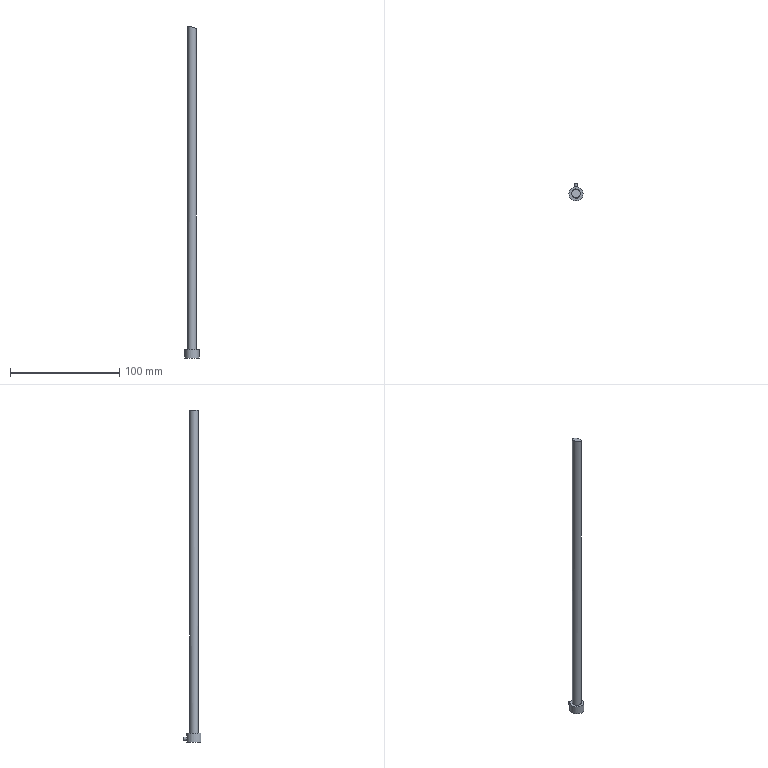Part | STEP file | E108-07-310 | 1 solid | 8 faces | box 13 x 16.5 x 303.697 mm | volume 15889 mm3 | cylinder 3 | plane 3 | spline 1 | cone 1 | commonest cylinder face diameters 3 x1 8 x1 13 x1
STEP:
#1=CARTESIAN_POINT('',(0.,0.,0.));
#2=DIRECTION('',(0.,0.,1.));
#3=DIRECTION('',(1.,0.,0.));
#4=AXIS2_PLACEMENT_3D('',#1,#2,#3);
#5=CARTESIAN_POINT('',(3.981,0.3919,301.273));
#6=VERTEX_POINT('',#5);
#7=CARTESIAN_POINT('',(3.981,0.3919,301.273));
#8=CARTESIAN_POINT('',(3.938,0.8228,301.273));
#9=CARTESIAN_POINT('',(3.823,1.252,301.297));
#10=CARTESIAN_POINT('',(3.646,1.645,301.341));
#11=CARTESIAN_POINT('',(3.469,2.037,301.385));
#12=CARTESIAN_POINT('',(3.225,2.404,301.45));
#13=CARTESIAN_POINT('',(2.937,2.716,301.53));
#14=CARTESIAN_POINT('',(2.642,3.034,301.612));
#15=CARTESIAN_POINT('',(2.293,3.305,301.711));
#16=CARTESIAN_POINT('',(1.918,3.51,301.82));
#17=CARTESIAN_POINT('',(1.526,3.724,301.934));
#18=CARTESIAN_POINT('',(1.096,3.872,302.061));
#19=CARTESIAN_POINT('',(0.6599,3.945,302.191));
#20=CARTESIAN_POINT('',(0.2071,4.021,302.327));
#21=CARTESIAN_POINT('',(-0.2637,4.018,302.469));
#22=CARTESIAN_POINT('',(-0.7148,3.936,302.606));
#23=CARTESIAN_POINT('',(-1.175,3.852,302.747));
#24=CARTESIAN_POINT('',(-1.627,3.685,302.886));
#25=CARTESIAN_POINT('',(-2.032,3.445,303.013));
#26=CARTESIAN_POINT('',(-2.434,3.208,303.139));
#27=CARTESIAN_POINT('',(-2.802,2.893,303.257));
#28=CARTESIAN_POINT('',(-3.101,2.526,303.355));
#29=CARTESIAN_POINT('',(-3.39,2.171,303.45));
#30=CARTESIAN_POINT('',(-3.623,1.757,303.531));
#31=CARTESIAN_POINT('',(-3.776,1.319,303.588));
#32=CARTESIAN_POINT('',(-3.923,0.8987,303.643));
#33=CARTESIAN_POINT('',(-4.,0.4448,303.678));
#34=CARTESIAN_POINT('',(-4.,-0.003275,303.691));
#35=CARTESIAN_POINT('',(-4.,-0.4371,303.703));
#36=CARTESIAN_POINT('',(-3.927,-0.8775,303.695));
#37=CARTESIAN_POINT('',(-3.787,-1.287,303.666));
#38=CARTESIAN_POINT('',(-3.649,-1.694,303.637));
#39=CARTESIAN_POINT('',(-3.442,-2.081,303.588));
#40=CARTESIAN_POINT('',(-3.185,-2.42,303.522));
#41=CARTESIAN_POINT('',(-2.924,-2.764,303.455));
#42=CARTESIAN_POINT('',(-2.604,-3.066,303.369));
#43=CARTESIAN_POINT('',(-2.251,-3.306,303.272));
#44=CARTESIAN_POINT('',(-1.886,-3.555,303.171));
#45=CARTESIAN_POINT('',(-1.478,-3.743,303.055));
#46=CARTESIAN_POINT('',(-1.057,-3.858,302.932));
#47=CARTESIAN_POINT('',(-0.6196,-3.978,302.805));
#48=CARTESIAN_POINT('',(-0.1578,-4.022,302.667));
#49=CARTESIAN_POINT('',(0.2919,-3.989,302.53));
#50=CARTESIAN_POINT('',(0.7551,-3.955,302.389));
#51=CARTESIAN_POINT('',(1.218,-3.838,302.245));
#52=CARTESIAN_POINT('',(1.643,-3.647,302.109));
#53=CARTESIAN_POINT('',(2.07,-3.454,301.973));
#54=CARTESIAN_POINT('',(2.471,-3.181,301.842));
#55=CARTESIAN_POINT('',(2.809,-2.848,301.729));
#56=CARTESIAN_POINT('',(3.138,-2.523,301.618));
#57=CARTESIAN_POINT('',(3.417,-2.131,301.52));
#58=CARTESIAN_POINT('',(3.618,-1.706,301.445));
#59=CARTESIAN_POINT('',(3.81,-1.3,301.374));
#60=CARTESIAN_POINT('',(3.935,-0.8505,301.322));
#61=CARTESIAN_POINT('',(3.98,-0.3986,301.295));
#62=CARTESIAN_POINT('',(4.006,-0.1368,301.28));
#63=CARTESIAN_POINT('',(4.007,0.1295,301.272));
#64=CARTESIAN_POINT('',(3.981,0.3919,301.273));
#65=B_SPLINE_CURVE_WITH_KNOTS('',3,(#7,#8,#9,#10,#11,#12,#13,#14,#15,#16,#17,#18,#19,#20,#21,#22,#23,#24,#25,#26,#27,#28,#29,#30,#31,#32,#33,#34,#35,#36,#37,#38,#39,#40,#41,#42,#43,#44,#45,#46,#47,#48,#49,#50,#51,#52,#53,#54,#55,#56,#57,#58,#59,#60,#61,#62,#63,#64),.UNSPECIFIED.,.T.,.F.,(1,3,3,3,3,3,3,3,3,3,3,3,3,3,3,3,3,3,3,3,3,1),(-0.03062,0.,0.05078,0.1015,0.1532,0.2072,0.2634,0.3207,0.3774,0.4324,0.485,0.5359,0.5863,0.6375,0.6906,0.7458,0.8028,0.8601,0.916,0.9694,1.,1.051),.UNSPECIFIED.);
#66=CARTESIAN_POINT('',(0.,0.,108.));
#67=DIRECTION('',(0.,0.,-1.));
#68=DIRECTION('',(-1.,0.,0.));
#69=AXIS2_PLACEMENT_3D('',#66,#67,#68);
#70=CYLINDRICAL_SURFACE('',#69,4.);
#71=CARTESIAN_POINT('',(9.327,-193.273));
#72=CARTESIAN_POINT('',(9.302,-193.273));
#73=CARTESIAN_POINT('',(9.254,-193.275));
#74=CARTESIAN_POINT('',(9.181,-193.286));
#75=CARTESIAN_POINT('',(9.108,-193.303));
#76=CARTESIAN_POINT('',(9.035,-193.327));
#77=CARTESIAN_POINT('',(8.962,-193.356));
#78=CARTESIAN_POINT('',(8.89,-193.392));
#79=CARTESIAN_POINT('',(8.817,-193.434));
#80=CARTESIAN_POINT('',(8.745,-193.481));
#81=CARTESIAN_POINT('',(8.674,-193.533));
#82=CARTESIAN_POINT('',(8.602,-193.589));
#83=CARTESIAN_POINT('',(8.53,-193.651));
#84=CARTESIAN_POINT('',(8.459,-193.716));
#85=CARTESIAN_POINT('',(8.388,-193.785));
#86=CARTESIAN_POINT('',(8.318,-193.857));
#87=CARTESIAN_POINT('',(8.247,-193.933));
#88=CARTESIAN_POINT('',(8.177,-194.011));
#89=CARTESIAN_POINT('',(8.106,-194.09));
#90=CARTESIAN_POINT('',(8.036,-194.172));
#91=CARTESIAN_POINT('',(7.966,-194.254));
#92=CARTESIAN_POINT('',(7.896,-194.338));
#93=CARTESIAN_POINT('',(7.826,-194.423));
#94=CARTESIAN_POINT('',(7.756,-194.507));
#95=CARTESIAN_POINT('',(7.687,-194.592));
#96=CARTESIAN_POINT('',(7.617,-194.675));
#97=CARTESIAN_POINT('',(7.547,-194.758));
#98=CARTESIAN_POINT('',(7.477,-194.839));
#99=CARTESIAN_POINT('',(7.406,-194.919));
#100=CARTESIAN_POINT('',(7.336,-194.997));
#101=CARTESIAN_POINT('',(7.266,-195.072));
#102=CARTESIAN_POINT('',(7.195,-195.145));
#103=CARTESIAN_POINT('',(7.124,-195.215));
#104=CARTESIAN_POINT('',(7.053,-195.281));
#105=CARTESIAN_POINT('',(6.982,-195.343));
#106=CARTESIAN_POINT('',(6.911,-195.401));
#107=CARTESIAN_POINT('',(6.839,-195.455));
#108=CARTESIAN_POINT('',(6.767,-195.504));
#109=CARTESIAN_POINT('',(6.695,-195.548));
#110=CARTESIAN_POINT('',(6.623,-195.587));
#111=CARTESIAN_POINT('',(6.55,-195.62));
#112=CARTESIAN_POINT('',(6.478,-195.648));
#113=CARTESIAN_POINT('',(6.405,-195.669));
#114=CARTESIAN_POINT('',(6.332,-195.685));
#115=CARTESIAN_POINT('',(6.259,-195.694));
#116=CARTESIAN_POINT('',(6.186,-195.698));
#117=CARTESIAN_POINT('',(6.113,-195.694));
#118=CARTESIAN_POINT('',(6.04,-195.685));
#119=CARTESIAN_POINT('',(5.967,-195.67));
#120=CARTESIAN_POINT('',(5.894,-195.648));
#121=CARTESIAN_POINT('',(5.821,-195.621));
#122=CARTESIAN_POINT('',(5.749,-195.587));
#123=CARTESIAN_POINT('',(5.676,-195.548));
#124=CARTESIAN_POINT('',(5.604,-195.504));
#125=CARTESIAN_POINT('',(5.532,-195.455));
#126=CARTESIAN_POINT('',(5.46,-195.4));
#127=CARTESIAN_POINT('',(5.388,-195.342));
#128=CARTESIAN_POINT('',(5.317,-195.279));
#129=CARTESIAN_POINT('',(5.246,-195.213));
#130=CARTESIAN_POINT('',(5.175,-195.142));
#131=CARTESIAN_POINT('',(5.104,-195.069));
#132=CARTESIAN_POINT('',(5.034,-194.993));
#133=CARTESIAN_POINT('',(4.964,-194.914));
#134=CARTESIAN_POINT('',(4.894,-194.834));
#135=CARTESIAN_POINT('',(4.823,-194.752));
#136=CARTESIAN_POINT('',(4.753,-194.668));
#137=CARTESIAN_POINT('',(4.683,-194.584));
#138=CARTESIAN_POINT('',(4.614,-194.499));
#139=CARTESIAN_POINT('',(4.544,-194.414));
#140=CARTESIAN_POINT('',(4.474,-194.329));
#141=CARTESIAN_POINT('',(4.404,-194.245));
#142=CARTESIAN_POINT('',(4.334,-194.162));
#143=CARTESIAN_POINT('',(4.264,-194.081));
#144=CARTESIAN_POINT('',(4.194,-194.001));
#145=CARTESIAN_POINT('',(4.124,-193.923));
#146=CARTESIAN_POINT('',(4.053,-193.848));
#147=CARTESIAN_POINT('',(3.982,-193.775));
#148=CARTESIAN_POINT('',(3.912,-193.707));
#149=CARTESIAN_POINT('',(3.841,-193.642));
#150=CARTESIAN_POINT('',(3.769,-193.581));
#151=CARTESIAN_POINT('',(3.697,-193.525));
#152=CARTESIAN_POINT('',(3.626,-193.473));
#153=CARTESIAN_POINT('',(3.554,-193.427));
#154=CARTESIAN_POINT('',(3.482,-193.386));
#155=CARTESIAN_POINT('',(3.409,-193.351));
#156=CARTESIAN_POINT('',(3.336,-193.322));
#157=CARTESIAN_POINT('',(3.264,-193.3));
#158=CARTESIAN_POINT('',(3.191,-193.284));
#159=CARTESIAN_POINT('',(3.117,-193.274));
#160=CARTESIAN_POINT('',(3.068,-193.272));
#161=CARTESIAN_POINT('',(3.043,-193.273));
#162=B_SPLINE_CURVE_WITH_KNOTS('',3,(#71,#72,#73,#74,#75,#76,#77,#78,#79,#80,#81,#82,#83,#84,#85,#86,#87,#88,#89,#90,#91,#92,#93,#94,#95,#96,#97,#98,#99,#100,#101,#102,#103,#104,#105,#106,#107,#108,#109,#110,#111,#112,#113,#114,#115,#116,#117,#118,#119,#120,#121,#122,#123,#124,#125,#126,#127,#128,#129,#130,#131,#132,#133,#134,#135,#136,#137,#138,#139,#140,#141,#142,#143,#144,#145,#146,#147,#148,#149,#150,#151,#152,#153,#154,#155,#156,#157,#158,#159,#160,#161),.UNSPECIFIED.,.F.,.F.,(4,1,1,1,1,1,1,1,1,1,1,1,1,1,1,1,1,1,1,1,1,1,1,1,1,1,1,1,1,1,1,1,1,1,1,1,1,1,1,1,1,1,1,1,1,1,1,1,1,1,1,1,1,1,1,1,1,1,1,1,1,1,1,1,1,1,1,1,1,1,1,1,1,1,1,1,1,1,1,1,1,1,1,1,1,1,1,1,4),(0.,0.01136,0.02273,0.03409,0.04545,0.05682,0.06818,0.07955,0.09091,0.1023,0.1136,0.125,0.1364,0.1477,0.1591,0.1705,0.1818,0.1932,0.2045,0.2159,0.2273,0.2386,0.25,0.2614,0.2727,0.2841,0.2955,0.3068,0.3182,0.3295,0.3409,0.3523,0.3636,0.375,0.3864,0.3977,0.4091,0.4205,0.4318,0.4432,0.4545,0.4659,0.4773,0.4886,0.5,0.5114,0.5227,0.5341,0.5455,0.5568,0.5682,0.5795,0.5909,0.6023,0.6136,0.625,0.6364,0.6477,0.6591,0.6705,0.6818,0.6932,0.7045,0.7159,0.7273,0.7386,0.75,0.7614,0.7727,0.7841,0.7955,0.8068,0.8182,0.8295,0.8409,0.8523,0.8636,0.875,0.8864,0.8977,0.9091,0.9205,0.9318,0.9432,0.9545,0.9659,0.9773,0.9886,1.),.QUASI_UNIFORM_KNOTS.);
#163=(GEOMETRIC_REPRESENTATION_CONTEXT(2)PARAMETRIC_REPRESENTATION_CONTEXT()REPRESENTATION_CONTEXT('',''));
#164=DEFINITIONAL_REPRESENTATION('',(#162),#163);
#165=PCURVE('',#70,#164);
#166=CARTESIAN_POINT('',(-6.109,-7.078,304.502));
#167=CARTESIAN_POINT('',(0.04478,-7.075,302.741));
#168=CARTESIAN_POINT('',(6.281,-7.073,300.808));
#169=CARTESIAN_POINT('',(12.6,-7.07,298.708));
#170=CARTESIAN_POINT('',(-6.116,-2.697,304.38));
#171=CARTESIAN_POINT('',(0.03497,-2.695,302.621));
#172=CARTESIAN_POINT('',(6.268,-2.692,300.689));
#173=CARTESIAN_POINT('',(12.584,-2.69,298.591));
#174=CARTESIAN_POINT('',(-6.125,1.683,304.257));
#175=CARTESIAN_POINT('',(0.02251,1.686,302.499));
#176=CARTESIAN_POINT('',(6.253,1.688,300.569));
#177=CARTESIAN_POINT('',(12.566,1.691,298.472));
#178=CARTESIAN_POINT('',(-6.137,6.064,304.132));
#179=CARTESIAN_POINT('',(0.007422,6.066,302.376));
#180=CARTESIAN_POINT('',(6.235,6.069,300.447));
#181=CARTESIAN_POINT('',(12.544,6.071,298.352));
#182=B_SPLINE_SURFACE_WITH_KNOTS('',3,3,((#166,#167,#168,#169),(#170,#171,#172,#173),(#174,#175,#176,#177),(#178,#179,#180,#181)),.UNSPECIFIED.,.F.,.F.,.F.,(4,4),(4,4),(0.,1.),(0.,1.),.PIECEWISE_BEZIER_KNOTS.);
#183=CARTESIAN_POINT('',(0.5681,0.5438));
#184=CARTESIAN_POINT('',(0.5754,0.5433));
#185=CARTESIAN_POINT('',(0.5901,0.5419));
#186=CARTESIAN_POINT('',(0.6119,0.5387));
#187=CARTESIAN_POINT('',(0.6333,0.5345));
#188=CARTESIAN_POINT('',(0.6541,0.5291));
#189=CARTESIAN_POINT('',(0.6741,0.5228));
#190=CARTESIAN_POINT('',(0.6935,0.5154));
#191=CARTESIAN_POINT('',(0.7121,0.5071));
#192=CARTESIAN_POINT('',(0.7297,0.4978));
#193=CARTESIAN_POINT('',(0.7462,0.4878));
#194=CARTESIAN_POINT('',(0.7616,0.477));
#195=CARTESIAN_POINT('',(0.7758,0.4654));
#196=CARTESIAN_POINT('',(0.7888,0.4532));
#197=CARTESIAN_POINT('',(0.8005,0.4404));
#198=CARTESIAN_POINT('',(0.8108,0.4271));
#199=CARTESIAN_POINT('',(0.8197,0.4134));
#200=CARTESIAN_POINT('',(0.8272,0.3992));
#201=CARTESIAN_POINT('',(0.8333,0.3847));
#202=CARTESIAN_POINT('',(0.838,0.37));
#203=CARTESIAN_POINT('',(0.8411,0.3552));
#204=CARTESIAN_POINT('',(0.8427,0.3402));
#205=CARTESIAN_POINT('',(0.8429,0.3251));
#206=CARTESIAN_POINT('',(0.8416,0.3101));
#207=CARTESIAN_POINT('',(0.8388,0.2952));
#208=CARTESIAN_POINT('',(0.8345,0.2805));
#209=CARTESIAN_POINT('',(0.8288,0.266));
#210=CARTESIAN_POINT('',(0.8216,0.2517));
#211=CARTESIAN_POINT('',(0.8131,0.2378));
#212=CARTESIAN_POINT('',(0.8032,0.2243));
#213=CARTESIAN_POINT('',(0.792,0.2114));
#214=CARTESIAN_POINT('',(0.7794,0.199));
#215=CARTESIAN_POINT('',(0.7655,0.1872));
#216=CARTESIAN_POINT('',(0.7505,0.1761));
#217=CARTESIAN_POINT('',(0.7345,0.1657));
#218=CARTESIAN_POINT('',(0.7174,0.1563));
#219=CARTESIAN_POINT('',(0.6992,0.1476));
#220=CARTESIAN_POINT('',(0.6802,0.1398));
#221=CARTESIAN_POINT('',(0.6604,0.133));
#222=CARTESIAN_POINT('',(0.64,0.1272));
#223=CARTESIAN_POINT('',(0.6189,0.1225));
#224=CARTESIAN_POINT('',(0.5973,0.1189));
#225=CARTESIAN_POINT('',(0.5754,0.1164));
#226=CARTESIAN_POINT('',(0.5532,0.115));
#227=CARTESIAN_POINT('',(0.5311,0.1147));
#228=CARTESIAN_POINT('',(0.5089,0.1157));
#229=CARTESIAN_POINT('',(0.4868,0.1178));
#230=CARTESIAN_POINT('',(0.465,0.121));
#231=CARTESIAN_POINT('',(0.4437,0.1253));
#232=CARTESIAN_POINT('',(0.423,0.1307));
#233=CARTESIAN_POINT('',(0.4028,0.1371));
#234=CARTESIAN_POINT('',(0.3833,0.1446));
#235=CARTESIAN_POINT('',(0.3647,0.153));
#236=CARTESIAN_POINT('',(0.3472,0.1623));
#237=CARTESIAN_POINT('',(0.3306,0.1725));
#238=CARTESIAN_POINT('',(0.3151,0.1835));
#239=CARTESIAN_POINT('',(0.3009,0.1952));
#240=CARTESIAN_POINT('',(0.2879,0.2075));
#241=CARTESIAN_POINT('',(0.2762,0.2203));
#242=CARTESIAN_POINT('',(0.2659,0.2338));
#243=CARTESIAN_POINT('',(0.2569,0.2476));
#244=CARTESIAN_POINT('',(0.2494,0.2619));
#245=CARTESIAN_POINT('',(0.2434,0.2763));
#246=CARTESIAN_POINT('',(0.2388,0.2911));
#247=CARTESIAN_POINT('',(0.2357,0.306));
#248=CARTESIAN_POINT('',(0.234,0.321));
#249=CARTESIAN_POINT('',(0.2339,0.3361));
#250=CARTESIAN_POINT('',(0.2352,0.351));
#251=CARTESIAN_POINT('',(0.2381,0.3658));
#252=CARTESIAN_POINT('',(0.2424,0.3806));
#253=CARTESIAN_POINT('',(0.2481,0.3951));
#254=CARTESIAN_POINT('',(0.2553,0.4092));
#255=CARTESIAN_POINT('',(0.2638,0.4229));
#256=CARTESIAN_POINT('',(0.2737,0.4363));
#257=CARTESIAN_POINT('',(0.285,0.4491));
#258=CARTESIAN_POINT('',(0.2975,0.4614));
#259=CARTESIAN_POINT('',(0.3113,0.4731));
#260=CARTESIAN_POINT('',(0.3262,0.484));
#261=CARTESIAN_POINT('',(0.3422,0.4943));
#262=CARTESIAN_POINT('',(0.3594,0.5037));
#263=CARTESIAN_POINT('',(0.3775,0.5123));
#264=CARTESIAN_POINT('',(0.3965,0.52));
#265=CARTESIAN_POINT('',(0.4162,0.5267));
#266=CARTESIAN_POINT('',(0.4367,0.5324));
#267=CARTESIAN_POINT('',(0.4578,0.5371));
#268=CARTESIAN_POINT('',(0.4794,0.5407));
#269=CARTESIAN_POINT('',(0.5012,0.5433));
#270=CARTESIAN_POINT('',(0.5234,0.5446));
#271=CARTESIAN_POINT('',(0.5458,0.5449));
#272=CARTESIAN_POINT('',(0.5607,0.5443));
#273=CARTESIAN_POINT('',(0.5681,0.5438));
#274=B_SPLINE_CURVE_WITH_KNOTS('',3,(#183,#184,#185,#186,#187,#188,#189,#190,#191,#192,#193,#194,#195,#196,#197,#198,#199,#200,#201,#202,#203,#204,#205,#206,#207,#208,#209,#210,#211,#212,#213,#214,#215,#216,#217,#218,#219,#220,#221,#222,#223,#224,#225,#226,#227,#228,#229,#230,#231,#232,#233,#234,#235,#236,#237,#238,#239,#240,#241,#242,#243,#244,#245,#246,#247,#248,#249,#250,#251,#252,#253,#254,#255,#256,#257,#258,#259,#260,#261,#262,#263,#264,#265,#266,#267,#268,#269,#270,#271,#272,#273),.UNSPECIFIED.,.T.,.F.,(4,1,1,1,1,1,1,1,1,1,1,1,1,1,1,1,1,1,1,1,1,1,1,1,1,1,1,1,1,1,1,1,1,1,1,1,1,1,1,1,1,1,1,1,1,1,1,1,1,1,1,1,1,1,1,1,1,1,1,1,1,1,1,1,1,1,1,1,1,1,1,1,1,1,1,1,1,1,1,1,1,1,1,1,1,1,1,1,4),(0.,0.01136,0.02273,0.03409,0.04545,0.05682,0.06818,0.07955,0.09091,0.1023,0.1136,0.125,0.1364,0.1477,0.1591,0.1705,0.1818,0.1932,0.2045,0.2159,0.2273,0.2386,0.25,0.2614,0.2727,0.2841,0.2955,0.3068,0.3182,0.3295,0.3409,0.3523,0.3636,0.375,0.3864,0.3977,0.4091,0.4205,0.4318,0.4432,0.4545,0.4659,0.4773,0.4886,0.5,0.5114,0.5227,0.5341,0.5455,0.5568,0.5682,0.5795,0.5909,0.6023,0.6136,0.625,0.6364,0.6477,0.6591,0.6705,0.6818,0.6932,0.7045,0.7159,0.7273,0.7386,0.75,0.7614,0.7727,0.7841,0.7955,0.8068,0.8182,0.8295,0.8409,0.8523,0.8636,0.875,0.8864,0.8977,0.9091,0.9205,0.9318,0.9432,0.9545,0.9659,0.9773,0.9886,1.),.QUASI_UNIFORM_KNOTS.);
#275=(GEOMETRIC_REPRESENTATION_CONTEXT(2)PARAMETRIC_REPRESENTATION_CONTEXT()REPRESENTATION_CONTEXT('',''));
#276=DEFINITIONAL_REPRESENTATION('',(#274),#275);
#277=PCURVE('',#182,#276);
#278=SURFACE_CURVE('',#65,(#165,#277),.PCURVE_S1.);
#279=EDGE_CURVE('',#6,#6,#278,.T.);
#280=ORIENTED_EDGE('',*,*,#279,.F.);
#281=CARTESIAN_POINT('',(3.981,0.3919,8.));
#282=VERTEX_POINT('',#281);
#283=CARTESIAN_POINT('',(3.981,0.3919,301.273));
#284=CARTESIAN_POINT('',(3.981,0.3919,8.));
#285=B_SPLINE_CURVE_WITH_KNOTS('',1,(#283,#284),.UNSPECIFIED.,.F.,.F.,(2,2),(-193.273,100.),.PIECEWISE_BEZIER_KNOTS.);
#286=CARTESIAN_POINT('',(9.327,0.));
#287=DIRECTION('',(0.,1.));
#288=VECTOR('',#287,1.);
#289=LINE('',#286,#288);
#290=(GEOMETRIC_REPRESENTATION_CONTEXT(2)PARAMETRIC_REPRESENTATION_CONTEXT()REPRESENTATION_CONTEXT('',''));
#291=DEFINITIONAL_REPRESENTATION('',(#289),#290);
#292=PCURVE('',#70,#291);
#293=CARTESIAN_POINT('',(3.043,0.));
#294=DIRECTION('',(0.,1.));
#295=VECTOR('',#294,1.);
#296=LINE('',#293,#295);
#297=(GEOMETRIC_REPRESENTATION_CONTEXT(2)PARAMETRIC_REPRESENTATION_CONTEXT()REPRESENTATION_CONTEXT('',''));
#298=DEFINITIONAL_REPRESENTATION('',(#296),#297);
#299=PCURVE('',#70,#298);
#300=SEAM_CURVE('',#285,(#292,#299),.PCURVE_S1.);
#301=EDGE_CURVE('',#6,#282,#300,.T.);
#302=ORIENTED_EDGE('',*,*,#301,.T.);
#303=CARTESIAN_POINT('',(4.,0.,8.));
#304=VERTEX_POINT('',#303);
#305=CARTESIAN_POINT('',(0.,0.,8.));
#306=DIRECTION('',(0.,0.,1.));
#307=DIRECTION('',(1.,0.,0.));
#308=AXIS2_PLACEMENT_3D('',#305,#306,#307);
#309=CIRCLE('',#308,4.);
#310=CARTESIAN_POINT('',(9.425,100.));
#311=DIRECTION('',(-1.,0.));
#312=VECTOR('',#311,1.);
#313=LINE('',#310,#312);
#314=(GEOMETRIC_REPRESENTATION_CONTEXT(2)PARAMETRIC_REPRESENTATION_CONTEXT()REPRESENTATION_CONTEXT('',''));
#315=DEFINITIONAL_REPRESENTATION('',(#313),#314);
#316=PCURVE('',#70,#315);
#317=CARTESIAN_POINT('',(0.,0.,8.));
#318=DIRECTION('',(0.,0.,-1.));
#319=DIRECTION('',(1.,0.,0.));
#320=AXIS2_PLACEMENT_3D('',#317,#318,#319);
#321=PLANE('',#320);
#322=CARTESIAN_POINT('',(4.,0.));
#323=CARTESIAN_POINT('',(4.,-6.928));
#324=CARTESIAN_POINT('',(-2.,-3.464));
#325=CARTESIAN_POINT('',(-8.,0.));
#326=CARTESIAN_POINT('',(-2.,3.464));
#327=CARTESIAN_POINT('',(4.,6.928));
#328=CARTESIAN_POINT('',(4.,0.));
#329=(BOUNDED_CURVE()B_SPLINE_CURVE(2,(#322,#323,#324,#325,#326,#327,#328),.UNSPECIFIED.,.T.,.F.)B_SPLINE_CURVE_WITH_KNOTS((1,2,2,2,2,1),(-2.094,0.,2.094,4.189,6.283,8.378),.UNSPECIFIED.)CURVE()GEOMETRIC_REPRESENTATION_ITEM()RATIONAL_B_SPLINE_CURVE((1.,0.5,1.,0.5,1.,0.5,1.))REPRESENTATION_ITEM(''));
#330=(GEOMETRIC_REPRESENTATION_CONTEXT(2)PARAMETRIC_REPRESENTATION_CONTEXT()REPRESENTATION_CONTEXT('',''));
#331=DEFINITIONAL_REPRESENTATION('',(#329),#330);
#332=PCURVE('',#321,#331);
#333=SURFACE_CURVE('',#309,(#316,#332),.PCURVE_S1.);
#334=EDGE_CURVE('',#282,#304,#333,.T.);
#335=ORIENTED_EDGE('',*,*,#334,.T.);
#336=CARTESIAN_POINT('',(0.,0.,8.));
#337=DIRECTION('',(0.,0.,1.));
#338=DIRECTION('',(1.,0.,0.));
#339=AXIS2_PLACEMENT_3D('',#336,#337,#338);
#340=CIRCLE('',#339,4.);
#341=CARTESIAN_POINT('',(3.142,100.));
#342=DIRECTION('',(-1.,0.));
#343=VECTOR('',#342,1.);
#344=LINE('',#341,#343);
#345=(GEOMETRIC_REPRESENTATION_CONTEXT(2)PARAMETRIC_REPRESENTATION_CONTEXT()REPRESENTATION_CONTEXT('',''));
#346=DEFINITIONAL_REPRESENTATION('',(#344),#345);
#347=PCURVE('',#70,#346);
#348=CARTESIAN_POINT('',(4.,0.));
#349=CARTESIAN_POINT('',(4.,-6.928));
#350=CARTESIAN_POINT('',(-2.,-3.464));
#351=CARTESIAN_POINT('',(-8.,0.));
#352=CARTESIAN_POINT('',(-2.,3.464));
#353=CARTESIAN_POINT('',(4.,6.928));
#354=CARTESIAN_POINT('',(4.,0.));
#355=(BOUNDED_CURVE()B_SPLINE_CURVE(2,(#348,#349,#350,#351,#352,#353,#354),.UNSPECIFIED.,.T.,.F.)B_SPLINE_CURVE_WITH_KNOTS((1,2,2,2,2,1),(-2.094,0.,2.094,4.189,6.283,8.378),.UNSPECIFIED.)CURVE()GEOMETRIC_REPRESENTATION_ITEM()RATIONAL_B_SPLINE_CURVE((1.,0.5,1.,0.5,1.,0.5,1.))REPRESENTATION_ITEM(''));
#356=(GEOMETRIC_REPRESENTATION_CONTEXT(2)PARAMETRIC_REPRESENTATION_CONTEXT()REPRESENTATION_CONTEXT('',''));
#357=DEFINITIONAL_REPRESENTATION('',(#355),#356);
#358=PCURVE('',#321,#357);
#359=SURFACE_CURVE('',#340,(#347,#358),.PCURVE_S1.);
#360=EDGE_CURVE('',#304,#282,#359,.T.);
#361=ORIENTED_EDGE('',*,*,#360,.T.);
#362=ORIENTED_EDGE('',*,*,#301,.F.);
#363=EDGE_LOOP('',(#280,#302,#335,#361,#362));
#364=FACE_BOUND('',#363,.T.);
#365=ADVANCED_FACE('',(#364),#70,.T.);
#366=ORIENTED_EDGE('',*,*,#279,.F.);
#367=EDGE_LOOP('',(#366));
#368=FACE_BOUND('',#367,.F.);
#369=ADVANCED_FACE('',(#368),#182,.F.);
#370=CARTESIAN_POINT('',(6.5,0.,0.));
#371=VERTEX_POINT('',#370);
#372=CARTESIAN_POINT('',(-6.5,0.,0.));
#373=VERTEX_POINT('',#372);
#374=CARTESIAN_POINT('',(0.,0.,0.));
#375=DIRECTION('',(0.,0.,-1.));
#376=DIRECTION('',(-1.,0.,0.));
#377=AXIS2_PLACEMENT_3D('',#374,#375,#376);
#378=CIRCLE('',#377,6.5);
#379=CARTESIAN_POINT('',(0.,0.,8.));
#380=DIRECTION('',(0.,0.,-1.));
#381=DIRECTION('',(1.,0.,0.));
#382=AXIS2_PLACEMENT_3D('',#379,#380,#381);
#383=CYLINDRICAL_SURFACE('',#382,6.5);
#384=CARTESIAN_POINT('',(-3.142,8.));
#385=DIRECTION('',(1.,0.));
#386=VECTOR('',#385,1.);
#387=LINE('',#384,#386);
#388=(GEOMETRIC_REPRESENTATION_CONTEXT(2)PARAMETRIC_REPRESENTATION_CONTEXT()REPRESENTATION_CONTEXT('',''));
#389=DEFINITIONAL_REPRESENTATION('',(#387),#388);
#390=PCURVE('',#383,#389);
#391=CARTESIAN_POINT('',(240.,-1000.,0.));
#392=DIRECTION('',(0.,0.,1.));
#393=DIRECTION('',(-1.,0.,0.));
#394=AXIS2_PLACEMENT_3D('',#391,#392,#393);
#395=PLANE('',#394);
#396=CARTESIAN_POINT('',(246.5,-1000.));
#397=CARTESIAN_POINT('',(246.5,-1011.258));
#398=CARTESIAN_POINT('',(236.75,-1005.629));
#399=CARTESIAN_POINT('',(227.,-1000.));
#400=CARTESIAN_POINT('',(236.75,-994.371));
#401=CARTESIAN_POINT('',(246.5,-988.742));
#402=CARTESIAN_POINT('',(246.5,-1000.));
#403=(BOUNDED_CURVE()B_SPLINE_CURVE(2,(#396,#397,#398,#399,#400,#401,#402),.UNSPECIFIED.,.T.,.F.)B_SPLINE_CURVE_WITH_KNOTS((1,2,2,2,2,1),(-2.094,0.,2.094,4.189,6.283,8.378),.UNSPECIFIED.)CURVE()GEOMETRIC_REPRESENTATION_ITEM()RATIONAL_B_SPLINE_CURVE((1.,0.5,1.,0.5,1.,0.5,1.))REPRESENTATION_ITEM(''));
#404=(GEOMETRIC_REPRESENTATION_CONTEXT(2)PARAMETRIC_REPRESENTATION_CONTEXT()REPRESENTATION_CONTEXT('',''));
#405=DEFINITIONAL_REPRESENTATION('',(#403),#404);
#406=PCURVE('',#395,#405);
#407=SURFACE_CURVE('',#378,(#390,#406),.PCURVE_S1.);
#408=EDGE_CURVE('',#371,#373,#407,.T.);
#409=ORIENTED_EDGE('',*,*,#408,.F.);
#410=CARTESIAN_POINT('',(6.5,0.,8.));
#411=VERTEX_POINT('',#410);
#412=CARTESIAN_POINT('',(6.5,0.,8.));
#413=CARTESIAN_POINT('',(6.5,0.,0.));
#414=B_SPLINE_CURVE_WITH_KNOTS('',1,(#412,#413),.UNSPECIFIED.,.F.,.F.,(2,2),(0.,8.),.PIECEWISE_BEZIER_KNOTS.);
#415=CARTESIAN_POINT('',(0.,0.));
#416=DIRECTION('',(0.,1.));
#417=VECTOR('',#416,1.);
#418=LINE('',#415,#417);
#419=(GEOMETRIC_REPRESENTATION_CONTEXT(2)PARAMETRIC_REPRESENTATION_CONTEXT()REPRESENTATION_CONTEXT('',''));
#420=DEFINITIONAL_REPRESENTATION('',(#418),#419);
#421=PCURVE('',#383,#420);
#422=CARTESIAN_POINT('',(6.283,0.));
#423=DIRECTION('',(0.,1.));
#424=VECTOR('',#423,1.);
#425=LINE('',#422,#424);
#426=(GEOMETRIC_REPRESENTATION_CONTEXT(2)PARAMETRIC_REPRESENTATION_CONTEXT()REPRESENTATION_CONTEXT('',''));
#427=DEFINITIONAL_REPRESENTATION('',(#425),#426);
#428=PCURVE('',#383,#427);
#429=SEAM_CURVE('',#414,(#421,#428),.PCURVE_S1.);
#430=EDGE_CURVE('',#411,#371,#429,.T.);
#431=ORIENTED_EDGE('',*,*,#430,.F.);
#432=CARTESIAN_POINT('',(0.,0.,8.));
#433=DIRECTION('',(0.,0.,-1.));
#434=DIRECTION('',(1.,0.,0.));
#435=AXIS2_PLACEMENT_3D('',#432,#433,#434);
#436=CIRCLE('',#435,6.5);
#437=CARTESIAN_POINT('',(0.,0.));
#438=DIRECTION('',(1.,0.));
#439=VECTOR('',#438,1.);
#440=LINE('',#437,#439);
#441=(GEOMETRIC_REPRESENTATION_CONTEXT(2)PARAMETRIC_REPRESENTATION_CONTEXT()REPRESENTATION_CONTEXT('',''));
#442=DEFINITIONAL_REPRESENTATION('',(#440),#441);
#443=PCURVE('',#383,#442);
#444=CARTESIAN_POINT('',(0.,0.));
#445=DIRECTION('',(1.,0.));
#446=AXIS2_PLACEMENT_2D('',#444,#445);
#447=CIRCLE('',#446,6.5);
#448=(GEOMETRIC_REPRESENTATION_CONTEXT(2)PARAMETRIC_REPRESENTATION_CONTEXT()REPRESENTATION_CONTEXT('',''));
#449=DEFINITIONAL_REPRESENTATION('',(#447),#448);
#450=PCURVE('',#321,#449);
#451=SURFACE_CURVE('',#436,(#443,#450),.PCURVE_S1.);
#452=EDGE_CURVE('',#411,#411,#451,.T.);
#453=ORIENTED_EDGE('',*,*,#452,.T.);
#454=ORIENTED_EDGE('',*,*,#430,.T.);
#455=CARTESIAN_POINT('',(0.,0.,0.));
#456=DIRECTION('',(0.,0.,-1.));
#457=DIRECTION('',(-1.,0.,0.));
#458=AXIS2_PLACEMENT_3D('',#455,#456,#457);
#459=CIRCLE('',#458,6.5);
#460=CARTESIAN_POINT('',(3.142,8.));
#461=DIRECTION('',(1.,0.));
#462=VECTOR('',#461,1.);
#463=LINE('',#460,#462);
#464=(GEOMETRIC_REPRESENTATION_CONTEXT(2)PARAMETRIC_REPRESENTATION_CONTEXT()REPRESENTATION_CONTEXT('',''));
#465=DEFINITIONAL_REPRESENTATION('',(#463),#464);
#466=PCURVE('',#383,#465);
#467=CARTESIAN_POINT('',(246.5,-1000.));
#468=CARTESIAN_POINT('',(246.5,-1011.258));
#469=CARTESIAN_POINT('',(236.75,-1005.629));
#470=CARTESIAN_POINT('',(227.,-1000.));
#471=CARTESIAN_POINT('',(236.75,-994.371));
#472=CARTESIAN_POINT('',(246.5,-988.742));
#473=CARTESIAN_POINT('',(246.5,-1000.));
#474=(BOUNDED_CURVE()B_SPLINE_CURVE(2,(#467,#468,#469,#470,#471,#472,#473),.UNSPECIFIED.,.T.,.F.)B_SPLINE_CURVE_WITH_KNOTS((1,2,2,2,2,1),(-2.094,0.,2.094,4.189,6.283,8.378),.UNSPECIFIED.)CURVE()GEOMETRIC_REPRESENTATION_ITEM()RATIONAL_B_SPLINE_CURVE((1.,0.5,1.,0.5,1.,0.5,1.))REPRESENTATION_ITEM(''));
#475=(GEOMETRIC_REPRESENTATION_CONTEXT(2)PARAMETRIC_REPRESENTATION_CONTEXT()REPRESENTATION_CONTEXT('',''));
#476=DEFINITIONAL_REPRESENTATION('',(#474),#475);
#477=PCURVE('',#395,#476);
#478=SURFACE_CURVE('',#459,(#466,#477),.PCURVE_S1.);
#479=EDGE_CURVE('',#373,#371,#478,.T.);
#480=ORIENTED_EDGE('',*,*,#479,.F.);
#481=EDGE_LOOP('',(#409,#431,#453,#454,#480));
#482=FACE_BOUND('',#481,.T.);
#483=CARTESIAN_POINT('',(0.,6.5,1.5));
#484=VERTEX_POINT('',#483);
#485=CARTESIAN_POINT('',(0.,6.5,1.5));
#486=CARTESIAN_POINT('',(0.1654,6.5,1.5));
#487=CARTESIAN_POINT('',(0.3332,6.493,1.528));
#488=CARTESIAN_POINT('',(0.4892,6.482,1.582));
#489=CARTESIAN_POINT('',(0.6451,6.47,1.636));
#490=CARTESIAN_POINT('',(0.7936,6.453,1.717));
#491=CARTESIAN_POINT('',(0.9231,6.434,1.818));
#492=CARTESIAN_POINT('',(1.055,6.415,1.92));
#493=CARTESIAN_POINT('',(1.17,6.394,2.047));
#494=CARTESIAN_POINT('',(1.261,6.377,2.187));
#495=CARTESIAN_POINT('',(1.352,6.358,2.329));
#496=CARTESIAN_POINT('',(1.421,6.343,2.49));
#497=CARTESIAN_POINT('',(1.46,6.334,2.655));
#498=CARTESIAN_POINT('',(1.498,6.325,2.817));
#499=CARTESIAN_POINT('',(1.509,6.322,2.989));
#500=CARTESIAN_POINT('',(1.492,6.326,3.155));
#501=CARTESIAN_POINT('',(1.475,6.33,3.318));
#502=CARTESIAN_POINT('',(1.431,6.341,3.48));
#503=CARTESIAN_POINT('',(1.362,6.356,3.628));
#504=CARTESIAN_POINT('',(1.293,6.37,3.777));
#505=CARTESIAN_POINT('',(1.199,6.39,3.917));
#506=CARTESIAN_POINT('',(1.085,6.409,4.035));
#507=CARTESIAN_POINT('',(0.9695,6.428,4.157));
#508=CARTESIAN_POINT('',(0.8309,6.448,4.26));
#509=CARTESIAN_POINT('',(0.6809,6.464,4.337));
#510=CARTESIAN_POINT('',(0.5305,6.48,4.413));
#511=CARTESIAN_POINT('',(0.3642,6.492,4.465));
#512=CARTESIAN_POINT('',(0.1962,6.497,4.487));
#513=CARTESIAN_POINT('',(0.03191,6.502,4.509));
#514=CARTESIAN_POINT('',(-0.1386,6.501,4.503));
#515=CARTESIAN_POINT('',(-0.3008,6.493,4.47));
#516=CARTESIAN_POINT('',(-0.4611,6.486,4.437));
#517=CARTESIAN_POINT('',(-0.6177,6.472,4.377));
#518=CARTESIAN_POINT('',(-0.7583,6.456,4.294));
#519=CARTESIAN_POINT('',(-0.9011,6.439,4.211));
#520=CARTESIAN_POINT('',(-1.031,6.419,4.102));
#521=CARTESIAN_POINT('',(-1.139,6.399,3.976));
#522=CARTESIAN_POINT('',(-1.249,6.38,3.848));
#523=CARTESIAN_POINT('',(-1.338,6.361,3.699));
#524=CARTESIAN_POINT('',(-1.399,6.348,3.541));
#525=CARTESIAN_POINT('',(-1.46,6.334,3.384));
#526=CARTESIAN_POINT('',(-1.494,6.326,3.214));
#527=CARTESIAN_POINT('',(-1.499,6.325,3.046));
#528=CARTESIAN_POINT('',(-1.504,6.324,2.881));
#529=CARTESIAN_POINT('',(-1.482,6.329,2.714));
#530=CARTESIAN_POINT('',(-1.433,6.34,2.557));
#531=CARTESIAN_POINT('',(-1.385,6.351,2.4));
#532=CARTESIAN_POINT('',(-1.309,6.367,2.25));
#533=CARTESIAN_POINT('',(-1.214,6.386,2.119));
#534=CARTESIAN_POINT('',(-1.116,6.404,1.984));
#535=CARTESIAN_POINT('',(-0.9937,6.425,1.864));
#536=CARTESIAN_POINT('',(-0.8569,6.443,1.769));
#537=CARTESIAN_POINT('',(-0.7182,6.462,1.672));
#538=CARTESIAN_POINT('',(-0.5604,6.478,1.598));
#539=CARTESIAN_POINT('',(-0.3967,6.488,1.553));
#540=CARTESIAN_POINT('',(-0.2682,6.496,1.518));
#541=CARTESIAN_POINT('',(-0.1335,6.5,1.5));
#542=CARTESIAN_POINT('',(0.,6.5,1.5));
#543=B_SPLINE_CURVE_WITH_KNOTS('',3,(#485,#486,#487,#488,#489,#490,#491,#492,#493,#494,#495,#496,#497,#498,#499,#500,#501,#502,#503,#504,#505,#506,#507,#508,#509,#510,#511,#512,#513,#514,#515,#516,#517,#518,#519,#520,#521,#522,#523,#524,#525,#526,#527,#528,#529,#530,#531,#532,#533,#534,#535,#536,#537,#538,#539,#540,#541,#542),.UNSPECIFIED.,.T.,.F.,(1,3,3,3,3,3,3,3,3,3,3,3,3,3,3,3,3,3,3,3,3,1),(-0.04234,0.,0.05275,0.1054,0.159,0.2132,0.2665,0.3187,0.3713,0.4252,0.4793,0.5321,0.5843,0.6373,0.6915,0.7453,0.7978,0.85,0.9034,0.9577,1.,1.053),.UNSPECIFIED.);
#544=CARTESIAN_POINT('',(4.712,6.5));
#545=CARTESIAN_POINT('',(4.718,6.5));
#546=CARTESIAN_POINT('',(4.729,6.497));
#547=CARTESIAN_POINT('',(4.745,6.486));
#548=CARTESIAN_POINT('',(4.762,6.467));
#549=CARTESIAN_POINT('',(4.778,6.44));
#550=CARTESIAN_POINT('',(4.793,6.406));
#551=CARTESIAN_POINT('',(4.809,6.365));
#552=CARTESIAN_POINT('',(4.823,6.317));
#553=CARTESIAN_POINT('',(4.838,6.262));
#554=CARTESIAN_POINT('',(4.851,6.201));
#555=CARTESIAN_POINT('',(4.864,6.135));
#556=CARTESIAN_POINT('',(4.876,6.062));
#557=CARTESIAN_POINT('',(4.888,5.983));
#558=CARTESIAN_POINT('',(4.898,5.9));
#559=CARTESIAN_POINT('',(4.908,5.813));
#560=CARTESIAN_POINT('',(4.916,5.721));
#561=CARTESIAN_POINT('',(4.924,5.625));
#562=CARTESIAN_POINT('',(4.93,5.526));
#563=CARTESIAN_POINT('',(4.936,5.424));
#564=CARTESIAN_POINT('',(4.94,5.321));
#565=CARTESIAN_POINT('',(4.943,5.215));
#566=CARTESIAN_POINT('',(4.945,5.108));
#567=CARTESIAN_POINT('',(4.945,5.));
#568=CARTESIAN_POINT('',(4.945,4.893));
#569=CARTESIAN_POINT('',(4.943,4.787));
#570=CARTESIAN_POINT('',(4.94,4.681));
#571=CARTESIAN_POINT('',(4.936,4.576));
#572=CARTESIAN_POINT('',(4.93,4.474));
#573=CARTESIAN_POINT('',(4.924,4.376));
#574=CARTESIAN_POINT('',(4.916,4.28));
#575=CARTESIAN_POINT('',(4.908,4.188));
#576=CARTESIAN_POINT('',(4.898,4.1));
#577=CARTESIAN_POINT('',(4.888,4.017));
#578=CARTESIAN_POINT('',(4.877,3.939));
#579=CARTESIAN_POINT('',(4.864,3.866));
#580=CARTESIAN_POINT('',(4.851,3.799));
#581=CARTESIAN_POINT('',(4.838,3.738));
#582=CARTESIAN_POINT('',(4.824,3.683));
#583=CARTESIAN_POINT('',(4.809,3.635));
#584=CARTESIAN_POINT('',(4.793,3.594));
#585=CARTESIAN_POINT('',(4.778,3.56));
#586=CARTESIAN_POINT('',(4.762,3.533));
#587=CARTESIAN_POINT('',(4.745,3.514));
#588=CARTESIAN_POINT('',(4.729,3.503));
#589=CARTESIAN_POINT('',(4.713,3.499));
#590=CARTESIAN_POINT('',(4.696,3.503));
#591=CARTESIAN_POINT('',(4.679,3.514));
#592=CARTESIAN_POINT('',(4.663,3.533));
#593=CARTESIAN_POINT('',(4.647,3.56));
#594=CARTESIAN_POINT('',(4.632,3.594));
#595=CARTESIAN_POINT('',(4.616,3.635));
#596=CARTESIAN_POINT('',(4.601,3.683));
#597=CARTESIAN_POINT('',(4.587,3.737));
#598=CARTESIAN_POINT('',(4.574,3.798));
#599=CARTESIAN_POINT('',(4.561,3.865));
#600=CARTESIAN_POINT('',(4.548,3.938));
#601=CARTESIAN_POINT('',(4.537,4.016));
#602=CARTESIAN_POINT('',(4.527,4.099));
#603=CARTESIAN_POINT('',(4.517,4.187));
#604=CARTESIAN_POINT('',(4.508,4.279));
#605=CARTESIAN_POINT('',(4.501,4.375));
#606=CARTESIAN_POINT('',(4.494,4.473));
#607=CARTESIAN_POINT('',(4.489,4.575));
#608=CARTESIAN_POINT('',(4.485,4.679));
#609=CARTESIAN_POINT('',(4.482,4.785));
#610=CARTESIAN_POINT('',(4.48,4.892));
#611=CARTESIAN_POINT('',(4.479,4.999));
#612=CARTESIAN_POINT('',(4.48,5.106));
#613=CARTESIAN_POINT('',(4.482,5.213));
#614=CARTESIAN_POINT('',(4.485,5.319));
#615=CARTESIAN_POINT('',(4.489,5.423));
#616=CARTESIAN_POINT('',(4.494,5.524));
#617=CARTESIAN_POINT('',(4.501,5.624));
#618=CARTESIAN_POINT('',(4.508,5.72));
#619=CARTESIAN_POINT('',(4.517,5.812));
#620=CARTESIAN_POINT('',(4.526,5.899));
#621=CARTESIAN_POINT('',(4.537,5.982));
#622=CARTESIAN_POINT('',(4.548,6.061));
#623=CARTESIAN_POINT('',(4.56,6.134));
#624=CARTESIAN_POINT('',(4.573,6.201));
#625=CARTESIAN_POINT('',(4.587,6.262));
#626=CARTESIAN_POINT('',(4.601,6.316));
#627=CARTESIAN_POINT('',(4.616,6.364));
#628=CARTESIAN_POINT('',(4.631,6.406));
#629=CARTESIAN_POINT('',(4.647,6.44));
#630=CARTESIAN_POINT('',(4.663,6.466));
#631=CARTESIAN_POINT('',(4.679,6.486));
#632=CARTESIAN_POINT('',(4.696,6.497));
#633=CARTESIAN_POINT('',(4.707,6.5));
#634=CARTESIAN_POINT('',(4.712,6.5));
#635=B_SPLINE_CURVE_WITH_KNOTS('',3,(#544,#545,#546,#547,#548,#549,#550,#551,#552,#553,#554,#555,#556,#557,#558,#559,#560,#561,#562,#563,#564,#565,#566,#567,#568,#569,#570,#571,#572,#573,#574,#575,#576,#577,#578,#579,#580,#581,#582,#583,#584,#585,#586,#587,#588,#589,#590,#591,#592,#593,#594,#595,#596,#597,#598,#599,#600,#601,#602,#603,#604,#605,#606,#607,#608,#609,#610,#611,#612,#613,#614,#615,#616,#617,#618,#619,#620,#621,#622,#623,#624,#625,#626,#627,#628,#629,#630,#631,#632,#633,#634),.UNSPECIFIED.,.T.,.F.,(4,1,1,1,1,1,1,1,1,1,1,1,1,1,1,1,1,1,1,1,1,1,1,1,1,1,1,1,1,1,1,1,1,1,1,1,1,1,1,1,1,1,1,1,1,1,1,1,1,1,1,1,1,1,1,1,1,1,1,1,1,1,1,1,1,1,1,1,1,1,1,1,1,1,1,1,1,1,1,1,1,1,1,1,1,1,1,1,4),(0.,0.01136,0.02273,0.03409,0.04545,0.05682,0.06818,0.07955,0.09091,0.1023,0.1136,0.125,0.1364,0.1477,0.1591,0.1705,0.1818,0.1932,0.2045,0.2159,0.2273,0.2386,0.25,0.2614,0.2727,0.2841,0.2955,0.3068,0.3182,0.3295,0.3409,0.3523,0.3636,0.375,0.3864,0.3977,0.4091,0.4205,0.4318,0.4432,0.4545,0.4659,0.4773,0.4886,0.5,0.5114,0.5227,0.5341,0.5455,0.5568,0.5682,0.5795,0.5909,0.6023,0.6136,0.625,0.6364,0.6477,0.6591,0.6705,0.6818,0.6932,0.7045,0.7159,0.7273,0.7386,0.75,0.7614,0.7727,0.7841,0.7955,0.8068,0.8182,0.8295,0.8409,0.8523,0.8636,0.875,0.8864,0.8977,0.9091,0.9205,0.9318,0.9432,0.9545,0.9659,0.9773,0.9886,1.),.QUASI_UNIFORM_KNOTS.);
#636=(GEOMETRIC_REPRESENTATION_CONTEXT(2)PARAMETRIC_REPRESENTATION_CONTEXT()REPRESENTATION_CONTEXT('',''));
#637=DEFINITIONAL_REPRESENTATION('',(#635),#636);
#638=PCURVE('',#383,#637);
#639=CARTESIAN_POINT('',(0.,2.,3.));
#640=DIRECTION('',(0.,1.,0.));
#641=DIRECTION('',(0.,0.,-1.));
#642=AXIS2_PLACEMENT_3D('',#639,#640,#641);
#643=CYLINDRICAL_SURFACE('',#642,1.5);
#644=CARTESIAN_POINT('',(6.283,4.5));
#645=CARTESIAN_POINT('',(6.259,4.5));
#646=CARTESIAN_POINT('',(6.212,4.499));
#647=CARTESIAN_POINT('',(6.14,4.497));
#648=CARTESIAN_POINT('',(6.068,4.492));
#649=CARTESIAN_POINT('',(5.997,4.486));
#650=CARTESIAN_POINT('',(5.926,4.479));
#651=CARTESIAN_POINT('',(5.854,4.47));
#652=CARTESIAN_POINT('',(5.783,4.46));
#653=CARTESIAN_POINT('',(5.711,4.449));
#654=CARTESIAN_POINT('',(5.64,4.438));
#655=CARTESIAN_POINT('',(5.569,4.425));
#656=CARTESIAN_POINT('',(5.498,4.413));
#657=CARTESIAN_POINT('',(5.427,4.4));
#658=CARTESIAN_POINT('',(5.355,4.388));
#659=CARTESIAN_POINT('',(5.284,4.376));
#660=CARTESIAN_POINT('',(5.213,4.365));
#661=CARTESIAN_POINT('',(5.142,4.355));
#662=CARTESIAN_POINT('',(5.07,4.346));
#663=CARTESIAN_POINT('',(4.999,4.338));
#664=CARTESIAN_POINT('',(4.928,4.332));
#665=CARTESIAN_POINT('',(4.856,4.328));
#666=CARTESIAN_POINT('',(4.784,4.325));
#667=CARTESIAN_POINT('',(4.713,4.324));
#668=CARTESIAN_POINT('',(4.641,4.325));
#669=CARTESIAN_POINT('',(4.57,4.328));
#670=CARTESIAN_POINT('',(4.498,4.332));
#671=CARTESIAN_POINT('',(4.426,4.339));
#672=CARTESIAN_POINT('',(4.355,4.346));
#673=CARTESIAN_POINT('',(4.283,4.355));
#674=CARTESIAN_POINT('',(4.212,4.365));
#675=CARTESIAN_POINT('',(4.141,4.376));
#676=CARTESIAN_POINT('',(4.07,4.388));
#677=CARTESIAN_POINT('',(3.998,4.4));
#678=CARTESIAN_POINT('',(3.927,4.413));
#679=CARTESIAN_POINT('',(3.856,4.425));
#680=CARTESIAN_POINT('',(3.785,4.437));
#681=CARTESIAN_POINT('',(3.714,4.449));
#682=CARTESIAN_POINT('',(3.642,4.46));
#683=CARTESIAN_POINT('',(3.571,4.47));
#684=CARTESIAN_POINT('',(3.5,4.479));
#685=CARTESIAN_POINT('',(3.428,4.486));
#686=CARTESIAN_POINT('',(3.357,4.492));
#687=CARTESIAN_POINT('',(3.285,4.497));
#688=CARTESIAN_POINT('',(3.214,4.499));
#689=CARTESIAN_POINT('',(3.142,4.5));
#690=CARTESIAN_POINT('',(3.07,4.499));
#691=CARTESIAN_POINT('',(2.999,4.497));
#692=CARTESIAN_POINT('',(2.927,4.492));
#693=CARTESIAN_POINT('',(2.856,4.486));
#694=CARTESIAN_POINT('',(2.784,4.479));
#695=CARTESIAN_POINT('',(2.713,4.47));
#696=CARTESIAN_POINT('',(2.641,4.46));
#697=CARTESIAN_POINT('',(2.57,4.449));
#698=CARTESIAN_POINT('',(2.499,4.438));
#699=CARTESIAN_POINT('',(2.428,4.425));
#700=CARTESIAN_POINT('',(2.357,4.413));
#701=CARTESIAN_POINT('',(2.285,4.4));
#702=CARTESIAN_POINT('',(2.215,4.388));
#703=CARTESIAN_POINT('',(2.143,4.376));
#704=CARTESIAN_POINT('',(2.072,4.365));
#705=CARTESIAN_POINT('',(2.,4.355));
#706=CARTESIAN_POINT('',(1.929,4.346));
#707=CARTESIAN_POINT('',(1.858,4.339));
#708=CARTESIAN_POINT('',(1.786,4.332));
#709=CARTESIAN_POINT('',(1.715,4.328));
#710=CARTESIAN_POINT('',(1.643,4.325));
#711=CARTESIAN_POINT('',(1.572,4.324));
#712=CARTESIAN_POINT('',(1.5,4.325));
#713=CARTESIAN_POINT('',(1.428,4.328));
#714=CARTESIAN_POINT('',(1.357,4.332));
#715=CARTESIAN_POINT('',(1.285,4.338));
#716=CARTESIAN_POINT('',(1.214,4.346));
#717=CARTESIAN_POINT('',(1.142,4.355));
#718=CARTESIAN_POINT('',(1.071,4.365));
#719=CARTESIAN_POINT('',(0.9995,4.376));
#720=CARTESIAN_POINT('',(0.9286,4.388));
#721=CARTESIAN_POINT('',(0.8575,4.4));
#722=CARTESIAN_POINT('',(0.7862,4.413));
#723=CARTESIAN_POINT('',(0.7149,4.425));
#724=CARTESIAN_POINT('',(0.6436,4.437));
#725=CARTESIAN_POINT('',(0.5728,4.449));
#726=CARTESIAN_POINT('',(0.5015,4.46));
#727=CARTESIAN_POINT('',(0.43,4.47));
#728=CARTESIAN_POINT('',(0.3585,4.479));
#729=CARTESIAN_POINT('',(0.2872,4.486));
#730=CARTESIAN_POINT('',(0.2157,4.492));
#731=CARTESIAN_POINT('',(0.1438,4.497));
#732=CARTESIAN_POINT('',(0.07178,4.499));
#733=CARTESIAN_POINT('',(0.02388,4.5));
#734=CARTESIAN_POINT('',(0.,4.5));
#735=B_SPLINE_CURVE_WITH_KNOTS('',3,(#644,#645,#646,#647,#648,#649,#650,#651,#652,#653,#654,#655,#656,#657,#658,#659,#660,#661,#662,#663,#664,#665,#666,#667,#668,#669,#670,#671,#672,#673,#674,#675,#676,#677,#678,#679,#680,#681,#682,#683,#684,#685,#686,#687,#688,#689,#690,#691,#692,#693,#694,#695,#696,#697,#698,#699,#700,#701,#702,#703,#704,#705,#706,#707,#708,#709,#710,#711,#712,#713,#714,#715,#716,#717,#718,#719,#720,#721,#722,#723,#724,#725,#726,#727,#728,#729,#730,#731,#732,#733,#734),.UNSPECIFIED.,.F.,.F.,(4,1,1,1,1,1,1,1,1,1,1,1,1,1,1,1,1,1,1,1,1,1,1,1,1,1,1,1,1,1,1,1,1,1,1,1,1,1,1,1,1,1,1,1,1,1,1,1,1,1,1,1,1,1,1,1,1,1,1,1,1,1,1,1,1,1,1,1,1,1,1,1,1,1,1,1,1,1,1,1,1,1,1,1,1,1,1,1,4),(0.,0.01136,0.02273,0.03409,0.04545,0.05682,0.06818,0.07955,0.09091,0.1023,0.1136,0.125,0.1364,0.1477,0.1591,0.1705,0.1818,0.1932,0.2045,0.2159,0.2273,0.2386,0.25,0.2614,0.2727,0.2841,0.2955,0.3068,0.3182,0.3295,0.3409,0.3523,0.3636,0.375,0.3864,0.3977,0.4091,0.4205,0.4318,0.4432,0.4545,0.4659,0.4773,0.4886,0.5,0.5114,0.5227,0.5341,0.5455,0.5568,0.5682,0.5795,0.5909,0.6023,0.6136,0.625,0.6364,0.6477,0.6591,0.6705,0.6818,0.6932,0.7045,0.7159,0.7273,0.7386,0.75,0.7614,0.7727,0.7841,0.7955,0.8068,0.8182,0.8295,0.8409,0.8523,0.8636,0.875,0.8864,0.8977,0.9091,0.9205,0.9318,0.9432,0.9545,0.9659,0.9773,0.9886,1.),.QUASI_UNIFORM_KNOTS.);
#736=(GEOMETRIC_REPRESENTATION_CONTEXT(2)PARAMETRIC_REPRESENTATION_CONTEXT()REPRESENTATION_CONTEXT('',''));
#737=DEFINITIONAL_REPRESENTATION('',(#735),#736);
#738=PCURVE('',#643,#737);
#739=SURFACE_CURVE('',#543,(#638,#738),.PCURVE_S1.);
#740=EDGE_CURVE('',#484,#484,#739,.T.);
#741=ORIENTED_EDGE('',*,*,#740,.T.);
#742=EDGE_LOOP('',(#741));
#743=FACE_BOUND('',#742,.T.);
#744=ADVANCED_FACE('',(#482,#743),#383,.T.);
#745=ORIENTED_EDGE('',*,*,#360,.F.);
#746=ORIENTED_EDGE('',*,*,#334,.F.);
#747=EDGE_LOOP('',(#745,#746));
#748=FACE_BOUND('',#747,.T.);
#749=ORIENTED_EDGE('',*,*,#452,.F.);
#750=EDGE_LOOP('',(#749));
#751=FACE_BOUND('',#750,.T.);
#752=ADVANCED_FACE('',(#748,#751),#321,.F.);
#753=ORIENTED_EDGE('',*,*,#479,.T.);
#754=ORIENTED_EDGE('',*,*,#408,.T.);
#755=EDGE_LOOP('',(#753,#754));
#756=FACE_BOUND('',#755,.T.);
#757=ADVANCED_FACE('',(#756),#395,.F.);
#758=CARTESIAN_POINT('',(0.,10.,1.75));
#759=VERTEX_POINT('',#758);
#760=CARTESIAN_POINT('',(0.,10.,3.));
#761=DIRECTION('',(0.,1.,0.));
#762=DIRECTION('',(0.,0.,-1.));
#763=AXIS2_PLACEMENT_3D('',#760,#761,#762);
#764=CIRCLE('',#763,1.25);
#765=CARTESIAN_POINT('',(0.,10.,3.));
#766=DIRECTION('',(0.,1.,0.));
#767=DIRECTION('',(0.,0.,-1.));
#768=AXIS2_PLACEMENT_3D('',#765,#766,#767);
#769=PLANE('',#768);
#770=CARTESIAN_POINT('',(0.,0.));
#771=DIRECTION('',(1.,0.));
#772=AXIS2_PLACEMENT_2D('',#770,#771);
#773=CIRCLE('',#772,1.25);
#774=(GEOMETRIC_REPRESENTATION_CONTEXT(2)PARAMETRIC_REPRESENTATION_CONTEXT()REPRESENTATION_CONTEXT('',''));
#775=DEFINITIONAL_REPRESENTATION('',(#773),#774);
#776=PCURVE('',#769,#775);
#777=CARTESIAN_POINT('',(0.,9.75,3.));
#778=DIRECTION('',(0.,-1.,0.));
#779=DIRECTION('',(0.,0.,1.));
#780=AXIS2_PLACEMENT_3D('',#777,#778,#779);
#781=CONICAL_SURFACE('',#780,1.5,0.7854);
#782=CARTESIAN_POINT('',(9.425,-0.25));
#783=DIRECTION('',(-1.,0.));
#784=VECTOR('',#783,1.);
#785=LINE('',#782,#784);
#786=(GEOMETRIC_REPRESENTATION_CONTEXT(2)PARAMETRIC_REPRESENTATION_CONTEXT()REPRESENTATION_CONTEXT('',''));
#787=DEFINITIONAL_REPRESENTATION('',(#785),#786);
#788=PCURVE('',#781,#787);
#789=SURFACE_CURVE('',#764,(#776,#788),.PCURVE_S1.);
#790=EDGE_CURVE('',#759,#759,#789,.T.);
#791=ORIENTED_EDGE('',*,*,#790,.T.);
#792=EDGE_LOOP('',(#791));
#793=FACE_BOUND('',#792,.T.);
#794=ADVANCED_FACE('',(#793),#769,.T.);
#795=ORIENTED_EDGE('',*,*,#790,.F.);
#796=CARTESIAN_POINT('',(0.,9.75,1.5));
#797=VERTEX_POINT('',#796);
#798=CARTESIAN_POINT('',(0.,10.,1.75));
#799=CARTESIAN_POINT('',(0.,9.75,1.5));
#800=B_SPLINE_CURVE_WITH_KNOTS('',1,(#798,#799),.UNSPECIFIED.,.F.,.F.,(2,2),(-0.3536,0.),.PIECEWISE_BEZIER_KNOTS.);
#801=CARTESIAN_POINT('',(9.425,0.));
#802=DIRECTION('',(0.,1.));
#803=VECTOR('',#802,1.);
#804=LINE('',#801,#803);
#805=(GEOMETRIC_REPRESENTATION_CONTEXT(2)PARAMETRIC_REPRESENTATION_CONTEXT()REPRESENTATION_CONTEXT('',''));
#806=DEFINITIONAL_REPRESENTATION('',(#804),#805);
#807=PCURVE('',#781,#806);
#808=CARTESIAN_POINT('',(3.142,0.));
#809=DIRECTION('',(0.,1.));
#810=VECTOR('',#809,1.);
#811=LINE('',#808,#810);
#812=(GEOMETRIC_REPRESENTATION_CONTEXT(2)PARAMETRIC_REPRESENTATION_CONTEXT()REPRESENTATION_CONTEXT('',''));
#813=DEFINITIONAL_REPRESENTATION('',(#811),#812);
#814=PCURVE('',#781,#813);
#815=SEAM_CURVE('',#800,(#807,#814),.PCURVE_S1.);
#816=EDGE_CURVE('',#759,#797,#815,.T.);
#817=ORIENTED_EDGE('',*,*,#816,.T.);
#818=CARTESIAN_POINT('',(0.,9.75,3.));
#819=DIRECTION('',(0.,-1.,0.));
#820=DIRECTION('',(0.,0.,-1.));
#821=AXIS2_PLACEMENT_3D('',#818,#819,#820);
#822=CIRCLE('',#821,1.5);
#823=CARTESIAN_POINT('',(3.142,0.));
#824=DIRECTION('',(1.,0.));
#825=VECTOR('',#824,1.);
#826=LINE('',#823,#825);
#827=(GEOMETRIC_REPRESENTATION_CONTEXT(2)PARAMETRIC_REPRESENTATION_CONTEXT()REPRESENTATION_CONTEXT('',''));
#828=DEFINITIONAL_REPRESENTATION('',(#826),#827);
#829=PCURVE('',#781,#828);
#830=CARTESIAN_POINT('',(6.283,7.75));
#831=DIRECTION('',(-1.,0.));
#832=VECTOR('',#831,1.);
#833=LINE('',#830,#832);
#834=(GEOMETRIC_REPRESENTATION_CONTEXT(2)PARAMETRIC_REPRESENTATION_CONTEXT()REPRESENTATION_CONTEXT('',''));
#835=DEFINITIONAL_REPRESENTATION('',(#833),#834);
#836=PCURVE('',#643,#835);
#837=SURFACE_CURVE('',#822,(#829,#836),.PCURVE_S1.);
#838=EDGE_CURVE('',#797,#797,#837,.T.);
#839=ORIENTED_EDGE('',*,*,#838,.F.);
#840=ORIENTED_EDGE('',*,*,#816,.F.);
#841=EDGE_LOOP('',(#795,#817,#839,#840));
#842=FACE_BOUND('',#841,.T.);
#843=ADVANCED_FACE('',(#842),#781,.T.);
#844=ORIENTED_EDGE('',*,*,#740,.F.);
#845=CARTESIAN_POINT('',(0.,6.5,1.5));
#846=CARTESIAN_POINT('',(0.,9.75,1.5));
#847=B_SPLINE_CURVE_WITH_KNOTS('',1,(#845,#846),.UNSPECIFIED.,.F.,.F.,(2,2),(4.5,7.75),.PIECEWISE_BEZIER_KNOTS.);
#848=CARTESIAN_POINT('',(6.283,0.));
#849=DIRECTION('',(0.,1.));
#850=VECTOR('',#849,1.);
#851=LINE('',#848,#850);
#852=(GEOMETRIC_REPRESENTATION_CONTEXT(2)PARAMETRIC_REPRESENTATION_CONTEXT()REPRESENTATION_CONTEXT('',''));
#853=DEFINITIONAL_REPRESENTATION('',(#851),#852);
#854=PCURVE('',#643,#853);
#855=CARTESIAN_POINT('',(0.,0.));
#856=DIRECTION('',(0.,1.));
#857=VECTOR('',#856,1.);
#858=LINE('',#855,#857);
#859=(GEOMETRIC_REPRESENTATION_CONTEXT(2)PARAMETRIC_REPRESENTATION_CONTEXT()REPRESENTATION_CONTEXT('',''));
#860=DEFINITIONAL_REPRESENTATION('',(#858),#859);
#861=PCURVE('',#643,#860);
#862=SEAM_CURVE('',#847,(#854,#861),.PCURVE_S1.);
#863=EDGE_CURVE('',#484,#797,#862,.T.);
#864=ORIENTED_EDGE('',*,*,#863,.T.);
#865=ORIENTED_EDGE('',*,*,#838,.T.);
#866=ORIENTED_EDGE('',*,*,#863,.F.);
#867=EDGE_LOOP('',(#844,#864,#865,#866));
#868=FACE_BOUND('',#867,.T.);
#869=ADVANCED_FACE('',(#868),#643,.T.);
#870=CLOSED_SHELL('',(#365,#369,#744,#752,#757,#794,#843,#869));
#871=MANIFOLD_SOLID_BREP('',#870);
#872=(LENGTH_UNIT()NAMED_UNIT(*)SI_UNIT(.MILLI.,.METRE.));
#873=UNCERTAINTY_MEASURE_WITH_UNIT(LENGTH_MEASURE(0.00005),#872,'','');
#874=(NAMED_UNIT(*)PLANE_ANGLE_UNIT()SI_UNIT($,.RADIAN.));
#875=(NAMED_UNIT(*)SI_UNIT($,.STERADIAN.)SOLID_ANGLE_UNIT());
#876=(GEOMETRIC_REPRESENTATION_CONTEXT(3)GLOBAL_UNCERTAINTY_ASSIGNED_CONTEXT((#873))GLOBAL_UNIT_ASSIGNED_CONTEXT((#872,#874,#875))REPRESENTATION_CONTEXT('',''));
#877=ADVANCED_BREP_SHAPE_REPRESENTATION('',(#4,#871),#876);